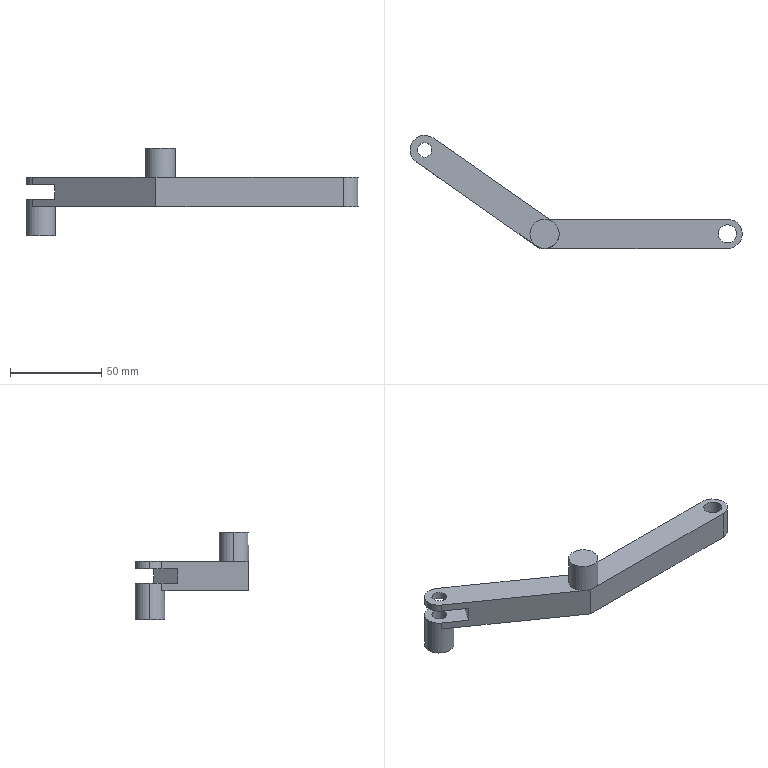Part | SolidWorks | features ICE 5, Extrusion 1 | 1 solid | 25 faces | box 181.532 x 61.886 x 48 mm | volume 50544 mm3 | cylinder 13 | plane 12 | commonest cylinder face diameters 16 x7 8 x4 10 x2
STEP:
#1=CARTESIAN_POINT('',(-169.532,45.886,12.));
#2=VERTEX_POINT('',#1);
#3=CARTESIAN_POINT('',(-161.532,45.886,12.));
#4=VERTEX_POINT('',#3);
#5=CARTESIAN_POINT('',(-165.532,45.886,12.));
#6=DIRECTION('',(0.,0.,1.));
#7=DIRECTION('',(1.,0.,0.));
#8=AXIS2_PLACEMENT_3D('',#5,#6,#7);
#9=CIRCLE('',#8,4.);
#10=EDGE_CURVE('',#2,#4,#9,.T.);
#11=ORIENTED_EDGE('',*,*,#10,.F.);
#12=CARTESIAN_POINT('',(-169.532,45.886,16.));
#13=VERTEX_POINT('',#12);
#14=CARTESIAN_POINT('',(-169.532,45.886,-22.));
#15=DIRECTION('',(0.,0.,1.));
#16=VECTOR('',#15,1000.);
#17=LINE('',#14,#16);
#18=EDGE_CURVE('',#2,#13,#17,.T.);
#19=ORIENTED_EDGE('',*,*,#18,.T.);
#20=CARTESIAN_POINT('',(-161.532,45.886,16.));
#21=VERTEX_POINT('',#20);
#22=CARTESIAN_POINT('',(-165.532,45.886,16.));
#23=DIRECTION('',(0.,0.,1.));
#24=DIRECTION('',(1.,0.,0.));
#25=AXIS2_PLACEMENT_3D('',#22,#23,#24);
#26=CIRCLE('',#25,4.);
#27=EDGE_CURVE('',#13,#21,#26,.T.);
#28=ORIENTED_EDGE('',*,*,#27,.T.);
#29=CARTESIAN_POINT('',(-161.532,45.886,-22.));
#30=DIRECTION('',(0.,0.,1.));
#31=VECTOR('',#30,1000.);
#32=LINE('',#29,#31);
#33=EDGE_CURVE('',#4,#21,#32,.T.);
#34=ORIENTED_EDGE('',*,*,#33,.F.);
#35=EDGE_LOOP('',(#11,#19,#28,#34));
#36=FACE_OUTER_BOUND('',#35,.T.);
#37=CARTESIAN_POINT('',(-165.532,45.886,-22.));
#38=DIRECTION('',(0.,0.,1.));
#39=DIRECTION('',(1.,0.,0.));
#40=AXIS2_PLACEMENT_3D('',#37,#38,#39);
#41=CYLINDRICAL_SURFACE('',#40,4.);
#42=ADVANCED_FACE('',(#36),#41,.F.);
#43=CARTESIAN_POINT('',(-169.532,45.886,-16.));
#44=VERTEX_POINT('',#43);
#45=CARTESIAN_POINT('',(-161.532,45.886,-16.));
#46=VERTEX_POINT('',#45);
#47=CARTESIAN_POINT('',(-165.532,45.886,-16.));
#48=DIRECTION('',(0.,0.,1.));
#49=DIRECTION('',(1.,0.,0.));
#50=AXIS2_PLACEMENT_3D('',#47,#48,#49);
#51=CIRCLE('',#50,4.);
#52=EDGE_CURVE('',#44,#46,#51,.T.);
#53=ORIENTED_EDGE('',*,*,#52,.F.);
#54=CARTESIAN_POINT('',(-169.532,45.886,4.));
#55=VERTEX_POINT('',#54);
#56=CARTESIAN_POINT('',(-169.532,45.886,-22.));
#57=DIRECTION('',(0.,0.,1.));
#58=VECTOR('',#57,1000.);
#59=LINE('',#56,#58);
#60=EDGE_CURVE('',#44,#55,#59,.T.);
#61=ORIENTED_EDGE('',*,*,#60,.T.);
#62=CARTESIAN_POINT('',(-161.532,45.886,4.));
#63=VERTEX_POINT('',#62);
#64=CARTESIAN_POINT('',(-165.532,45.886,4.));
#65=DIRECTION('',(0.,0.,-1.));
#66=DIRECTION('',(-1.,0.,0.));
#67=AXIS2_PLACEMENT_3D('',#64,#65,#66);
#68=CIRCLE('',#67,4.);
#69=EDGE_CURVE('',#63,#55,#68,.T.);
#70=ORIENTED_EDGE('',*,*,#69,.F.);
#71=CARTESIAN_POINT('',(-161.532,45.886,-22.));
#72=DIRECTION('',(0.,0.,1.));
#73=VECTOR('',#72,1000.);
#74=LINE('',#71,#73);
#75=EDGE_CURVE('',#46,#63,#74,.T.);
#76=ORIENTED_EDGE('',*,*,#75,.F.);
#77=EDGE_LOOP('',(#53,#61,#70,#76));
#78=FACE_OUTER_BOUND('',#77,.T.);
#79=CARTESIAN_POINT('',(-165.532,45.886,-22.));
#80=DIRECTION('',(0.,0.,1.));
#81=DIRECTION('',(1.,0.,0.));
#82=AXIS2_PLACEMENT_3D('',#79,#80,#81);
#83=CYLINDRICAL_SURFACE('',#82,4.);
#84=ADVANCED_FACE('',(#78),#83,.F.);
#85=CARTESIAN_POINT('',(-108.,0.,32.));
#86=VERTEX_POINT('',#85);
#87=CARTESIAN_POINT('',(-92.,0.,32.));
#88=VERTEX_POINT('',#87);
#89=CARTESIAN_POINT('',(-100.,0.,32.));
#90=DIRECTION('',(0.,0.,-1.));
#91=DIRECTION('',(-1.,0.,0.));
#92=AXIS2_PLACEMENT_3D('',#89,#90,#91);
#93=CIRCLE('',#92,8.);
#94=EDGE_CURVE('',#86,#88,#93,.T.);
#95=ORIENTED_EDGE('',*,*,#94,.T.);
#96=CARTESIAN_POINT('',(-92.,0.,16.));
#97=VERTEX_POINT('',#96);
#98=CARTESIAN_POINT('',(-92.,0.,32.));
#99=DIRECTION('',(0.,0.,-1.));
#100=VECTOR('',#99,1000.);
#101=LINE('',#98,#100);
#102=EDGE_CURVE('',#88,#97,#101,.T.);
#103=ORIENTED_EDGE('',*,*,#102,.T.);
#104=CARTESIAN_POINT('',(-108.,0.,16.));
#105=VERTEX_POINT('',#104);
#106=CARTESIAN_POINT('',(-100.,0.,16.));
#107=DIRECTION('',(0.,0.,-1.));
#108=DIRECTION('',(-1.,0.,0.));
#109=AXIS2_PLACEMENT_3D('',#106,#107,#108);
#110=CIRCLE('',#109,8.);
#111=EDGE_CURVE('',#105,#97,#110,.T.);
#112=ORIENTED_EDGE('',*,*,#111,.F.);
#113=CARTESIAN_POINT('',(-108.,0.,32.));
#114=DIRECTION('',(0.,0.,-1.));
#115=VECTOR('',#114,1000.);
#116=LINE('',#113,#115);
#117=EDGE_CURVE('',#86,#105,#116,.T.);
#118=ORIENTED_EDGE('',*,*,#117,.F.);
#119=EDGE_LOOP('',(#95,#103,#112,#118));
#120=FACE_OUTER_BOUND('',#119,.T.);
#121=CARTESIAN_POINT('',(-100.,0.,32.));
#122=DIRECTION('',(0.,0.,-1.));
#123=DIRECTION('',(-1.,0.,0.));
#124=AXIS2_PLACEMENT_3D('',#121,#122,#123);
#125=CYLINDRICAL_SURFACE('',#124,8.);
#126=ADVANCED_FACE('',(#120),#125,.T.);
#127=CARTESIAN_POINT('',(-5.,0.,0.));
#128=VERTEX_POINT('',#127);
#129=CARTESIAN_POINT('',(5.,0.,0.));
#130=VERTEX_POINT('',#129);
#131=CARTESIAN_POINT('',(0.,0.,0.));
#132=DIRECTION('',(0.,0.,1.));
#133=DIRECTION('',(1.,0.,0.));
#134=AXIS2_PLACEMENT_3D('',#131,#132,#133);
#135=CIRCLE('',#134,5.);
#136=EDGE_CURVE('',#128,#130,#135,.T.);
#137=ORIENTED_EDGE('',*,*,#136,.F.);
#138=CARTESIAN_POINT('',(-5.,0.,16.));
#139=VERTEX_POINT('',#138);
#140=CARTESIAN_POINT('',(-5.,0.,0.));
#141=DIRECTION('',(0.,0.,1.));
#142=VECTOR('',#141,1000.);
#143=LINE('',#140,#142);
#144=EDGE_CURVE('',#128,#139,#143,.T.);
#145=ORIENTED_EDGE('',*,*,#144,.T.);
#146=CARTESIAN_POINT('',(5.,0.,16.));
#147=VERTEX_POINT('',#146);
#148=CARTESIAN_POINT('',(0.,0.,16.));
#149=DIRECTION('',(0.,0.,1.));
#150=DIRECTION('',(1.,0.,0.));
#151=AXIS2_PLACEMENT_3D('',#148,#149,#150);
#152=CIRCLE('',#151,5.);
#153=EDGE_CURVE('',#139,#147,#152,.T.);
#154=ORIENTED_EDGE('',*,*,#153,.T.);
#155=CARTESIAN_POINT('',(5.,0.,0.));
#156=DIRECTION('',(0.,0.,1.));
#157=VECTOR('',#156,1000.);
#158=LINE('',#155,#157);
#159=EDGE_CURVE('',#130,#147,#158,.T.);
#160=ORIENTED_EDGE('',*,*,#159,.F.);
#161=EDGE_LOOP('',(#137,#145,#154,#160));
#162=FACE_OUTER_BOUND('',#161,.T.);
#163=CARTESIAN_POINT('',(0.,0.,0.));
#164=DIRECTION('',(0.,0.,1.));
#165=DIRECTION('',(1.,0.,0.));
#166=AXIS2_PLACEMENT_3D('',#163,#164,#165);
#167=CYLINDRICAL_SURFACE('',#166,5.);
#168=ADVANCED_FACE('',(#162),#167,.F.);
#169=CARTESIAN_POINT('',(-160.944,52.439,0.));
#170=VERTEX_POINT('',#169);
#171=CARTESIAN_POINT('',(-157.532,45.886,0.));
#172=VERTEX_POINT('',#171);
#173=CARTESIAN_POINT('',(-165.532,45.886,0.));
#174=DIRECTION('',(0.,0.,-1.));
#175=DIRECTION('',(-1.,0.,0.));
#176=AXIS2_PLACEMENT_3D('',#173,#174,#175);
#177=CIRCLE('',#176,8.);
#178=EDGE_CURVE('',#170,#172,#177,.T.);
#179=ORIENTED_EDGE('',*,*,#178,.T.);
#180=CARTESIAN_POINT('',(-157.532,45.886,-16.));
#181=VERTEX_POINT('',#180);
#182=CARTESIAN_POINT('',(-157.532,45.886,16.));
#183=DIRECTION('',(0.,0.,-1.));
#184=VECTOR('',#183,1000.);
#185=LINE('',#182,#184);
#186=EDGE_CURVE('',#172,#181,#185,.T.);
#187=ORIENTED_EDGE('',*,*,#186,.T.);
#188=CARTESIAN_POINT('',(-173.532,45.886,-16.));
#189=VERTEX_POINT('',#188);
#190=CARTESIAN_POINT('',(-165.532,45.886,-16.));
#191=DIRECTION('',(0.,0.,1.));
#192=DIRECTION('',(1.,0.,0.));
#193=AXIS2_PLACEMENT_3D('',#190,#191,#192);
#194=CIRCLE('',#193,8.);
#195=EDGE_CURVE('',#181,#189,#194,.T.);
#196=ORIENTED_EDGE('',*,*,#195,.T.);
#197=CARTESIAN_POINT('',(-173.532,45.886,4.));
#198=VERTEX_POINT('',#197);
#199=CARTESIAN_POINT('',(-173.532,45.886,16.));
#200=DIRECTION('',(0.,0.,-1.));
#201=VECTOR('',#200,1000.);
#202=LINE('',#199,#201);
#203=EDGE_CURVE('',#198,#189,#202,.T.);
#204=ORIENTED_EDGE('',*,*,#203,.F.);
#205=CARTESIAN_POINT('',(-160.944,52.439,4.));
#206=VERTEX_POINT('',#205);
#207=CARTESIAN_POINT('',(-165.532,45.886,4.));
#208=DIRECTION('',(0.,0.,-1.));
#209=DIRECTION('',(-1.,0.,0.));
#210=AXIS2_PLACEMENT_3D('',#207,#208,#209);
#211=CIRCLE('',#210,8.);
#212=EDGE_CURVE('',#198,#206,#211,.T.);
#213=ORIENTED_EDGE('',*,*,#212,.T.);
#214=CARTESIAN_POINT('',(-160.944,52.439,16.));
#215=DIRECTION('',(0.,0.,-1.));
#216=VECTOR('',#215,1000.);
#217=LINE('',#214,#216);
#218=EDGE_CURVE('',#206,#170,#217,.T.);
#219=ORIENTED_EDGE('',*,*,#218,.T.);
#220=EDGE_LOOP('',(#179,#187,#196,#204,#213,#219));
#221=FACE_OUTER_BOUND('',#220,.T.);
#222=CARTESIAN_POINT('',(-165.532,45.886,16.));
#223=DIRECTION('',(0.,0.,-1.));
#224=DIRECTION('',(-1.,0.,0.));
#225=AXIS2_PLACEMENT_3D('',#222,#223,#224);
#226=CYLINDRICAL_SURFACE('',#225,8.);
#227=ADVANCED_FACE('',(#221),#226,.T.);
#228=CARTESIAN_POINT('',(-173.532,45.886,16.));
#229=VERTEX_POINT('',#228);
#230=CARTESIAN_POINT('',(-170.121,39.333,16.));
#231=VERTEX_POINT('',#230);
#232=CARTESIAN_POINT('',(-165.532,45.886,16.));
#233=DIRECTION('',(0.,0.,1.));
#234=DIRECTION('',(1.,0.,0.));
#235=AXIS2_PLACEMENT_3D('',#232,#233,#234);
#236=CIRCLE('',#235,8.);
#237=EDGE_CURVE('',#229,#231,#236,.T.);
#238=ORIENTED_EDGE('',*,*,#237,.F.);
#239=CARTESIAN_POINT('',(-173.532,45.886,12.));
#240=VERTEX_POINT('',#239);
#241=CARTESIAN_POINT('',(-173.532,45.886,16.));
#242=DIRECTION('',(0.,0.,-1.));
#243=VECTOR('',#242,1000.);
#244=LINE('',#241,#243);
#245=EDGE_CURVE('',#229,#240,#244,.T.);
#246=ORIENTED_EDGE('',*,*,#245,.T.);
#247=CARTESIAN_POINT('',(-170.121,39.333,12.));
#248=VERTEX_POINT('',#247);
#249=CARTESIAN_POINT('',(-165.532,45.886,12.));
#250=DIRECTION('',(0.,0.,1.));
#251=DIRECTION('',(1.,0.,0.));
#252=AXIS2_PLACEMENT_3D('',#249,#250,#251);
#253=CIRCLE('',#252,8.);
#254=EDGE_CURVE('',#240,#248,#253,.T.);
#255=ORIENTED_EDGE('',*,*,#254,.T.);
#256=CARTESIAN_POINT('',(-170.121,39.333,16.));
#257=DIRECTION('',(0.,0.,-1.));
#258=VECTOR('',#257,1000.);
#259=LINE('',#256,#258);
#260=EDGE_CURVE('',#231,#248,#259,.T.);
#261=ORIENTED_EDGE('',*,*,#260,.F.);
#262=EDGE_LOOP('',(#238,#246,#255,#261));
#263=FACE_OUTER_BOUND('',#262,.T.);
#264=CARTESIAN_POINT('',(-165.532,45.886,16.));
#265=DIRECTION('',(0.,0.,-1.));
#266=DIRECTION('',(-1.,0.,0.));
#267=AXIS2_PLACEMENT_3D('',#264,#265,#266);
#268=CYLINDRICAL_SURFACE('',#267,8.);
#269=ADVANCED_FACE('',(#263),#268,.T.);
#270=ORIENTED_EDGE('',*,*,#245,.F.);
#271=CARTESIAN_POINT('',(-160.944,52.439,16.));
#272=VERTEX_POINT('',#271);
#273=CARTESIAN_POINT('',(-165.532,45.886,16.));
#274=DIRECTION('',(0.,0.,1.));
#275=DIRECTION('',(1.,0.,0.));
#276=AXIS2_PLACEMENT_3D('',#273,#274,#275);
#277=CIRCLE('',#276,8.);
#278=EDGE_CURVE('',#272,#229,#277,.T.);
#279=ORIENTED_EDGE('',*,*,#278,.F.);
#280=CARTESIAN_POINT('',(-160.944,52.439,12.));
#281=VERTEX_POINT('',#280);
#282=CARTESIAN_POINT('',(-160.944,52.439,16.));
#283=DIRECTION('',(0.,0.,-1.));
#284=VECTOR('',#283,1000.);
#285=LINE('',#282,#284);
#286=EDGE_CURVE('',#272,#281,#285,.T.);
#287=ORIENTED_EDGE('',*,*,#286,.T.);
#288=CARTESIAN_POINT('',(-165.532,45.886,12.));
#289=DIRECTION('',(0.,0.,1.));
#290=DIRECTION('',(1.,0.,0.));
#291=AXIS2_PLACEMENT_3D('',#288,#289,#290);
#292=CIRCLE('',#291,8.);
#293=EDGE_CURVE('',#281,#240,#292,.T.);
#294=ORIENTED_EDGE('',*,*,#293,.T.);
#295=EDGE_LOOP('',(#270,#279,#287,#294));
#296=FACE_OUTER_BOUND('',#295,.T.);
#297=CARTESIAN_POINT('',(-165.532,45.886,16.));
#298=DIRECTION('',(0.,0.,-1.));
#299=DIRECTION('',(-1.,0.,0.));
#300=AXIS2_PLACEMENT_3D('',#297,#298,#299);
#301=CYLINDRICAL_SURFACE('',#300,8.);
#302=ADVANCED_FACE('',(#296),#301,.T.);
#303=CARTESIAN_POINT('',(-102.522,-8.,16.));
#304=VERTEX_POINT('',#303);
#305=CARTESIAN_POINT('',(-100.,-8.,16.));
#306=VERTEX_POINT('',#305);
#307=CARTESIAN_POINT('',(0.,-8.,16.));
#308=DIRECTION('',(1.,0.,0.));
#309=VECTOR('',#308,1000.);
#310=LINE('',#307,#309);
#311=EDGE_CURVE('',#304,#306,#310,.T.);
#312=ORIENTED_EDGE('',*,*,#311,.T.);
#313=CARTESIAN_POINT('',(-104.589,-6.553,16.));
#314=VERTEX_POINT('',#313);
#315=CARTESIAN_POINT('',(-100.,0.,16.));
#316=DIRECTION('',(0.,0.,-1.));
#317=DIRECTION('',(-1.,0.,0.));
#318=AXIS2_PLACEMENT_3D('',#315,#316,#317);
#319=CIRCLE('',#318,8.);
#320=EDGE_CURVE('',#306,#314,#319,.T.);
#321=ORIENTED_EDGE('',*,*,#320,.T.);
#322=CARTESIAN_POINT('',(-102.522,-8.,16.));
#323=DIRECTION('',(0.8192,-0.5736,0.));
#324=VECTOR('',#323,1000.);
#325=LINE('',#322,#324);
#326=EDGE_CURVE('',#314,#304,#325,.T.);
#327=ORIENTED_EDGE('',*,*,#326,.T.);
#328=EDGE_LOOP('',(#312,#321,#327));
#329=FACE_OUTER_BOUND('',#328,.T.);
#330=CARTESIAN_POINT('',(0.,0.,16.));
#331=DIRECTION('',(0.,0.,-1.));
#332=DIRECTION('',(-1.,0.,0.));
#333=AXIS2_PLACEMENT_3D('',#330,#331,#332);
#334=PLANE('',#333);
#335=ADVANCED_FACE('',(#329),#334,.F.);
#336=CARTESIAN_POINT('',(0.,-8.,0.));
#337=VERTEX_POINT('',#336);
#338=CARTESIAN_POINT('',(0.,8.,0.));
#339=VERTEX_POINT('',#338);
#340=CARTESIAN_POINT('',(0.,0.,0.));
#341=DIRECTION('',(0.,0.,1.));
#342=DIRECTION('',(-1.,0.,0.));
#343=AXIS2_PLACEMENT_3D('',#340,#341,#342);
#344=CIRCLE('',#343,8.);
#345=EDGE_CURVE('',#337,#339,#344,.T.);
#346=ORIENTED_EDGE('',*,*,#345,.T.);
#347=CARTESIAN_POINT('',(0.,8.,16.));
#348=VERTEX_POINT('',#347);
#349=CARTESIAN_POINT('',(0.,8.,16.));
#350=DIRECTION('',(0.,0.,-1.));
#351=VECTOR('',#350,1000.);
#352=LINE('',#349,#351);
#353=EDGE_CURVE('',#348,#339,#352,.T.);
#354=ORIENTED_EDGE('',*,*,#353,.F.);
#355=CARTESIAN_POINT('',(0.,-8.,16.));
#356=VERTEX_POINT('',#355);
#357=CARTESIAN_POINT('',(0.,0.,16.));
#358=DIRECTION('',(0.,0.,1.));
#359=DIRECTION('',(-1.,0.,0.));
#360=AXIS2_PLACEMENT_3D('',#357,#358,#359);
#361=CIRCLE('',#360,8.);
#362=EDGE_CURVE('',#356,#348,#361,.T.);
#363=ORIENTED_EDGE('',*,*,#362,.F.);
#364=CARTESIAN_POINT('',(0.,-8.,16.));
#365=DIRECTION('',(0.,0.,-1.));
#366=VECTOR('',#365,1000.);
#367=LINE('',#364,#366);
#368=EDGE_CURVE('',#356,#337,#367,.T.);
#369=ORIENTED_EDGE('',*,*,#368,.T.);
#370=EDGE_LOOP('',(#346,#354,#363,#369));
#371=FACE_OUTER_BOUND('',#370,.T.);
#372=CARTESIAN_POINT('',(0.,0.,16.));
#373=DIRECTION('',(0.,0.,-1.));
#374=DIRECTION('',(-1.,0.,0.));
#375=AXIS2_PLACEMENT_3D('',#372,#373,#374);
#376=CYLINDRICAL_SURFACE('',#375,8.);
#377=ADVANCED_FACE('',(#371),#376,.T.);
#378=CARTESIAN_POINT('',(-97.478,8.,0.));
#379=VERTEX_POINT('',#378);
#380=CARTESIAN_POINT('',(0.,8.,0.));
#381=DIRECTION('',(-1.,0.,0.));
#382=VECTOR('',#381,1000.);
#383=LINE('',#380,#382);
#384=EDGE_CURVE('',#339,#379,#383,.T.);
#385=ORIENTED_EDGE('',*,*,#384,.T.);
#386=CARTESIAN_POINT('',(-97.478,8.,16.));
#387=VERTEX_POINT('',#386);
#388=CARTESIAN_POINT('',(-97.478,8.,16.));
#389=DIRECTION('',(0.,0.,-1.));
#390=VECTOR('',#389,1000.);
#391=LINE('',#388,#390);
#392=EDGE_CURVE('',#387,#379,#391,.T.);
#393=ORIENTED_EDGE('',*,*,#392,.F.);
#394=CARTESIAN_POINT('',(0.,8.,16.));
#395=DIRECTION('',(-1.,0.,0.));
#396=VECTOR('',#395,1000.);
#397=LINE('',#394,#396);
#398=EDGE_CURVE('',#348,#387,#397,.T.);
#399=ORIENTED_EDGE('',*,*,#398,.F.);
#400=ORIENTED_EDGE('',*,*,#353,.T.);
#401=EDGE_LOOP('',(#385,#393,#399,#400));
#402=FACE_OUTER_BOUND('',#401,.T.);
#403=CARTESIAN_POINT('',(0.,8.,16.));
#404=DIRECTION('',(0.,-1.,0.));
#405=DIRECTION('',(0.,0.,-1.));
#406=AXIS2_PLACEMENT_3D('',#403,#404,#405);
#407=PLANE('',#406);
#408=ADVANCED_FACE('',(#402),#407,.F.);
#409=CARTESIAN_POINT('',(-148.656,43.836,4.));
#410=VERTEX_POINT('',#409);
#411=CARTESIAN_POINT('',(-148.656,43.836,12.));
#412=VERTEX_POINT('',#411);
#413=CARTESIAN_POINT('',(-148.656,43.836,16.));
#414=DIRECTION('',(0.,0.,1.));
#415=VECTOR('',#414,1000.);
#416=LINE('',#413,#415);
#417=EDGE_CURVE('',#410,#412,#416,.T.);
#418=ORIENTED_EDGE('',*,*,#417,.T.);
#419=CARTESIAN_POINT('',(-97.478,8.,12.));
#420=DIRECTION('',(-0.8192,0.5736,0.));
#421=VECTOR('',#420,1000.);
#422=LINE('',#419,#421);
#423=EDGE_CURVE('',#412,#281,#422,.T.);
#424=ORIENTED_EDGE('',*,*,#423,.T.);
#425=ORIENTED_EDGE('',*,*,#286,.F.);
#426=CARTESIAN_POINT('',(-97.478,8.,16.));
#427=DIRECTION('',(-0.8192,0.5736,0.));
#428=VECTOR('',#427,1000.);
#429=LINE('',#426,#428);
#430=EDGE_CURVE('',#387,#272,#429,.T.);
#431=ORIENTED_EDGE('',*,*,#430,.F.);
#432=ORIENTED_EDGE('',*,*,#392,.T.);
#433=CARTESIAN_POINT('',(-97.478,8.,0.));
#434=DIRECTION('',(-0.8192,0.5736,0.));
#435=VECTOR('',#434,1000.);
#436=LINE('',#433,#435);
#437=EDGE_CURVE('',#379,#170,#436,.T.);
#438=ORIENTED_EDGE('',*,*,#437,.T.);
#439=ORIENTED_EDGE('',*,*,#218,.F.);
#440=CARTESIAN_POINT('',(-97.478,8.,4.));
#441=DIRECTION('',(0.8192,-0.5736,0.));
#442=VECTOR('',#441,1000.);
#443=LINE('',#440,#442);
#444=EDGE_CURVE('',#206,#410,#443,.T.);
#445=ORIENTED_EDGE('',*,*,#444,.T.);
#446=EDGE_LOOP('',(#418,#424,#425,#431,#432,#438,#439,#445));
#447=FACE_OUTER_BOUND('',#446,.T.);
#448=CARTESIAN_POINT('',(-97.478,8.,16.));
#449=DIRECTION('',(-0.5736,-0.8192,0.));
#450=DIRECTION('',(0.8192,-0.5736,0.));
#451=AXIS2_PLACEMENT_3D('',#448,#449,#450);
#452=PLANE('',#451);
#453=ADVANCED_FACE('',(#447),#452,.F.);
#454=ORIENTED_EDGE('',*,*,#186,.F.);
#455=CARTESIAN_POINT('',(-170.121,39.333,0.));
#456=VERTEX_POINT('',#455);
#457=CARTESIAN_POINT('',(-165.532,45.886,0.));
#458=DIRECTION('',(0.,0.,-1.));
#459=DIRECTION('',(-1.,0.,0.));
#460=AXIS2_PLACEMENT_3D('',#457,#458,#459);
#461=CIRCLE('',#460,8.);
#462=EDGE_CURVE('',#172,#456,#461,.T.);
#463=ORIENTED_EDGE('',*,*,#462,.T.);
#464=CARTESIAN_POINT('',(-170.121,39.333,4.));
#465=VERTEX_POINT('',#464);
#466=CARTESIAN_POINT('',(-170.121,39.333,16.));
#467=DIRECTION('',(0.,0.,-1.));
#468=VECTOR('',#467,1000.);
#469=LINE('',#466,#468);
#470=EDGE_CURVE('',#465,#456,#469,.T.);
#471=ORIENTED_EDGE('',*,*,#470,.F.);
#472=CARTESIAN_POINT('',(-165.532,45.886,4.));
#473=DIRECTION('',(0.,0.,-1.));
#474=DIRECTION('',(-1.,0.,0.));
#475=AXIS2_PLACEMENT_3D('',#472,#473,#474);
#476=CIRCLE('',#475,8.);
#477=EDGE_CURVE('',#465,#198,#476,.T.);
#478=ORIENTED_EDGE('',*,*,#477,.T.);
#479=ORIENTED_EDGE('',*,*,#203,.T.);
#480=CARTESIAN_POINT('',(-165.532,45.886,-16.));
#481=DIRECTION('',(0.,0.,1.));
#482=DIRECTION('',(1.,0.,0.));
#483=AXIS2_PLACEMENT_3D('',#480,#481,#482);
#484=CIRCLE('',#483,8.);
#485=EDGE_CURVE('',#189,#181,#484,.T.);
#486=ORIENTED_EDGE('',*,*,#485,.T.);
#487=EDGE_LOOP('',(#454,#463,#471,#478,#479,#486));
#488=FACE_OUTER_BOUND('',#487,.T.);
#489=CARTESIAN_POINT('',(-165.532,45.886,16.));
#490=DIRECTION('',(0.,0.,-1.));
#491=DIRECTION('',(-1.,0.,0.));
#492=AXIS2_PLACEMENT_3D('',#489,#490,#491);
#493=CYLINDRICAL_SURFACE('',#492,8.);
#494=ADVANCED_FACE('',(#488),#493,.T.);
#495=ORIENTED_EDGE('',*,*,#260,.T.);
#496=CARTESIAN_POINT('',(-157.833,30.729,12.));
#497=VERTEX_POINT('',#496);
#498=CARTESIAN_POINT('',(-157.833,30.729,12.));
#499=DIRECTION('',(-0.8192,0.5736,0.));
#500=VECTOR('',#499,1000.);
#501=LINE('',#498,#500);
#502=EDGE_CURVE('',#497,#248,#501,.T.);
#503=ORIENTED_EDGE('',*,*,#502,.F.);
#504=CARTESIAN_POINT('',(-157.833,30.729,4.));
#505=VERTEX_POINT('',#504);
#506=CARTESIAN_POINT('',(-157.833,30.729,4.));
#507=DIRECTION('',(0.,0.,1.));
#508=VECTOR('',#507,1000.);
#509=LINE('',#506,#508);
#510=EDGE_CURVE('',#505,#497,#509,.T.);
#511=ORIENTED_EDGE('',*,*,#510,.F.);
#512=CARTESIAN_POINT('',(-102.522,-8.,4.));
#513=DIRECTION('',(-0.8192,0.5736,0.));
#514=VECTOR('',#513,1000.);
#515=LINE('',#512,#514);
#516=EDGE_CURVE('',#505,#465,#515,.T.);
#517=ORIENTED_EDGE('',*,*,#516,.T.);
#518=ORIENTED_EDGE('',*,*,#470,.T.);
#519=CARTESIAN_POINT('',(-102.522,-8.,0.));
#520=VERTEX_POINT('',#519);
#521=CARTESIAN_POINT('',(-102.522,-8.,0.));
#522=DIRECTION('',(0.8192,-0.5736,0.));
#523=VECTOR('',#522,1000.);
#524=LINE('',#521,#523);
#525=EDGE_CURVE('',#456,#520,#524,.T.);
#526=ORIENTED_EDGE('',*,*,#525,.T.);
#527=CARTESIAN_POINT('',(-102.522,-8.,16.));
#528=DIRECTION('',(0.,0.,-1.));
#529=VECTOR('',#528,1000.);
#530=LINE('',#527,#529);
#531=EDGE_CURVE('',#304,#520,#530,.T.);
#532=ORIENTED_EDGE('',*,*,#531,.F.);
#533=ORIENTED_EDGE('',*,*,#326,.F.);
#534=CARTESIAN_POINT('',(-102.522,-8.,16.));
#535=DIRECTION('',(0.8192,-0.5736,0.));
#536=VECTOR('',#535,1000.);
#537=LINE('',#534,#536);
#538=EDGE_CURVE('',#231,#314,#537,.T.);
#539=ORIENTED_EDGE('',*,*,#538,.F.);
#540=EDGE_LOOP('',(#495,#503,#511,#517,#518,#526,#532,#533,#539));
#541=FACE_OUTER_BOUND('',#540,.T.);
#542=CARTESIAN_POINT('',(-102.522,-8.,16.));
#543=DIRECTION('',(0.5736,0.8192,0.));
#544=DIRECTION('',(-0.8192,0.5736,0.));
#545=AXIS2_PLACEMENT_3D('',#542,#543,#544);
#546=PLANE('',#545);
#547=ADVANCED_FACE('',(#541),#546,.F.);
#548=CARTESIAN_POINT('',(0.,-8.,16.));
#549=DIRECTION('',(1.,0.,0.));
#550=VECTOR('',#549,1000.);
#551=LINE('',#548,#550);
#552=EDGE_CURVE('',#306,#356,#551,.T.);
#553=ORIENTED_EDGE('',*,*,#552,.F.);
#554=ORIENTED_EDGE('',*,*,#311,.F.);
#555=ORIENTED_EDGE('',*,*,#531,.T.);
#556=CARTESIAN_POINT('',(0.,-8.,0.));
#557=DIRECTION('',(1.,0.,0.));
#558=VECTOR('',#557,1000.);
#559=LINE('',#556,#558);
#560=EDGE_CURVE('',#520,#337,#559,.T.);
#561=ORIENTED_EDGE('',*,*,#560,.T.);
#562=ORIENTED_EDGE('',*,*,#368,.F.);
#563=EDGE_LOOP('',(#553,#554,#555,#561,#562));
#564=FACE_OUTER_BOUND('',#563,.T.);
#565=CARTESIAN_POINT('',(0.,-8.,16.));
#566=DIRECTION('',(0.,1.,0.));
#567=DIRECTION('',(0.,0.,1.));
#568=AXIS2_PLACEMENT_3D('',#565,#566,#567);
#569=PLANE('',#568);
#570=ADVANCED_FACE('',(#564),#569,.F.);
#571=CARTESIAN_POINT('',(-165.532,45.886,16.));
#572=DIRECTION('',(0.,0.,1.));
#573=DIRECTION('',(1.,0.,0.));
#574=AXIS2_PLACEMENT_3D('',#571,#572,#573);
#575=CIRCLE('',#574,4.);
#576=EDGE_CURVE('',#21,#13,#575,.T.);
#577=ORIENTED_EDGE('',*,*,#576,.F.);
#578=ORIENTED_EDGE('',*,*,#27,.F.);
#579=EDGE_LOOP('',(#577,#578));
#580=FACE_BOUND('',#579,.T.);
#581=CARTESIAN_POINT('',(0.,0.,16.));
#582=DIRECTION('',(0.,0.,1.));
#583=DIRECTION('',(1.,0.,0.));
#584=AXIS2_PLACEMENT_3D('',#581,#582,#583);
#585=CIRCLE('',#584,5.);
#586=EDGE_CURVE('',#147,#139,#585,.T.);
#587=ORIENTED_EDGE('',*,*,#586,.F.);
#588=ORIENTED_EDGE('',*,*,#153,.F.);
#589=EDGE_LOOP('',(#587,#588));
#590=FACE_BOUND('',#589,.T.);
#591=ORIENTED_EDGE('',*,*,#430,.T.);
#592=ORIENTED_EDGE('',*,*,#278,.T.);
#593=ORIENTED_EDGE('',*,*,#237,.T.);
#594=ORIENTED_EDGE('',*,*,#538,.T.);
#595=CARTESIAN_POINT('',(-100.,0.,16.));
#596=DIRECTION('',(0.,0.,-1.));
#597=DIRECTION('',(-1.,0.,0.));
#598=AXIS2_PLACEMENT_3D('',#595,#596,#597);
#599=CIRCLE('',#598,8.);
#600=EDGE_CURVE('',#314,#105,#599,.T.);
#601=ORIENTED_EDGE('',*,*,#600,.T.);
#602=ORIENTED_EDGE('',*,*,#111,.T.);
#603=CARTESIAN_POINT('',(-100.,0.,16.));
#604=DIRECTION('',(0.,0.,-1.));
#605=DIRECTION('',(-1.,0.,0.));
#606=AXIS2_PLACEMENT_3D('',#603,#604,#605);
#607=CIRCLE('',#606,8.);
#608=EDGE_CURVE('',#97,#306,#607,.T.);
#609=ORIENTED_EDGE('',*,*,#608,.T.);
#610=ORIENTED_EDGE('',*,*,#552,.T.);
#611=ORIENTED_EDGE('',*,*,#362,.T.);
#612=ORIENTED_EDGE('',*,*,#398,.T.);
#613=EDGE_LOOP('',(#591,#592,#593,#594,#601,#602,#609,#610,#611,#612));
#614=FACE_OUTER_BOUND('',#613,.T.);
#615=CARTESIAN_POINT('',(0.,0.,16.));
#616=DIRECTION('',(0.,0.,-1.));
#617=DIRECTION('',(-1.,0.,0.));
#618=AXIS2_PLACEMENT_3D('',#615,#616,#617);
#619=PLANE('',#618);
#620=ADVANCED_FACE('',(#580,#590,#614),#619,.F.);
#621=ORIENTED_EDGE('',*,*,#178,.F.);
#622=ORIENTED_EDGE('',*,*,#437,.F.);
#623=ORIENTED_EDGE('',*,*,#384,.F.);
#624=ORIENTED_EDGE('',*,*,#345,.F.);
#625=ORIENTED_EDGE('',*,*,#560,.F.);
#626=ORIENTED_EDGE('',*,*,#525,.F.);
#627=ORIENTED_EDGE('',*,*,#462,.F.);
#628=EDGE_LOOP('',(#621,#622,#623,#624,#625,#626,#627));
#629=FACE_OUTER_BOUND('',#628,.T.);
#630=CARTESIAN_POINT('',(0.,0.,0.));
#631=DIRECTION('',(0.,0.,1.));
#632=DIRECTION('',(1.,0.,0.));
#633=AXIS2_PLACEMENT_3D('',#630,#631,#632);
#634=CIRCLE('',#633,5.);
#635=EDGE_CURVE('',#130,#128,#634,.T.);
#636=ORIENTED_EDGE('',*,*,#635,.T.);
#637=ORIENTED_EDGE('',*,*,#136,.T.);
#638=EDGE_LOOP('',(#636,#637));
#639=FACE_BOUND('',#638,.T.);
#640=CARTESIAN_POINT('',(0.,0.,0.));
#641=DIRECTION('',(0.,0.,-1.));
#642=DIRECTION('',(-1.,0.,0.));
#643=AXIS2_PLACEMENT_3D('',#640,#641,#642);
#644=PLANE('',#643);
#645=ADVANCED_FACE('',(#629,#639),#644,.T.);
#646=ORIENTED_EDGE('',*,*,#144,.F.);
#647=ORIENTED_EDGE('',*,*,#635,.F.);
#648=ORIENTED_EDGE('',*,*,#159,.T.);
#649=ORIENTED_EDGE('',*,*,#586,.T.);
#650=EDGE_LOOP('',(#646,#647,#648,#649));
#651=FACE_OUTER_BOUND('',#650,.T.);
#652=CARTESIAN_POINT('',(0.,0.,0.));
#653=DIRECTION('',(0.,0.,1.));
#654=DIRECTION('',(1.,0.,0.));
#655=AXIS2_PLACEMENT_3D('',#652,#653,#654);
#656=CYLINDRICAL_SURFACE('',#655,5.);
#657=ADVANCED_FACE('',(#651),#656,.F.);
#658=ORIENTED_EDGE('',*,*,#102,.F.);
#659=CARTESIAN_POINT('',(-100.,0.,32.));
#660=DIRECTION('',(0.,0.,-1.));
#661=DIRECTION('',(-1.,0.,0.));
#662=AXIS2_PLACEMENT_3D('',#659,#660,#661);
#663=CIRCLE('',#662,8.);
#664=EDGE_CURVE('',#88,#86,#663,.T.);
#665=ORIENTED_EDGE('',*,*,#664,.T.);
#666=ORIENTED_EDGE('',*,*,#117,.T.);
#667=ORIENTED_EDGE('',*,*,#600,.F.);
#668=ORIENTED_EDGE('',*,*,#320,.F.);
#669=ORIENTED_EDGE('',*,*,#608,.F.);
#670=EDGE_LOOP('',(#658,#665,#666,#667,#668,#669));
#671=FACE_OUTER_BOUND('',#670,.T.);
#672=CARTESIAN_POINT('',(-100.,0.,32.));
#673=DIRECTION('',(0.,0.,-1.));
#674=DIRECTION('',(-1.,0.,0.));
#675=AXIS2_PLACEMENT_3D('',#672,#673,#674);
#676=CYLINDRICAL_SURFACE('',#675,8.);
#677=ADVANCED_FACE('',(#671),#676,.T.);
#678=ORIENTED_EDGE('',*,*,#94,.F.);
#679=ORIENTED_EDGE('',*,*,#664,.F.);
#680=EDGE_LOOP('',(#678,#679));
#681=FACE_OUTER_BOUND('',#680,.T.);
#682=CARTESIAN_POINT('',(-100.,0.,32.));
#683=DIRECTION('',(0.,0.,-1.));
#684=DIRECTION('',(-1.,0.,0.));
#685=AXIS2_PLACEMENT_3D('',#682,#683,#684);
#686=PLANE('',#685);
#687=ADVANCED_FACE('',(#681),#686,.F.);
#688=CARTESIAN_POINT('',(-165.532,45.886,-16.));
#689=DIRECTION('',(0.,0.,1.));
#690=DIRECTION('',(1.,0.,0.));
#691=AXIS2_PLACEMENT_3D('',#688,#689,#690);
#692=CIRCLE('',#691,4.);
#693=EDGE_CURVE('',#46,#44,#692,.T.);
#694=ORIENTED_EDGE('',*,*,#693,.T.);
#695=ORIENTED_EDGE('',*,*,#52,.T.);
#696=EDGE_LOOP('',(#694,#695));
#697=FACE_BOUND('',#696,.T.);
#698=ORIENTED_EDGE('',*,*,#485,.F.);
#699=ORIENTED_EDGE('',*,*,#195,.F.);
#700=EDGE_LOOP('',(#698,#699));
#701=FACE_OUTER_BOUND('',#700,.T.);
#702=CARTESIAN_POINT('',(-165.532,45.886,-16.));
#703=DIRECTION('',(0.,0.,1.));
#704=DIRECTION('',(1.,0.,0.));
#705=AXIS2_PLACEMENT_3D('',#702,#703,#704);
#706=PLANE('',#705);
#707=ADVANCED_FACE('',(#697,#701),#706,.F.);
#708=CARTESIAN_POINT('',(-165.532,45.886,12.));
#709=DIRECTION('',(0.,0.,1.));
#710=DIRECTION('',(1.,0.,0.));
#711=AXIS2_PLACEMENT_3D('',#708,#709,#710);
#712=CIRCLE('',#711,4.);
#713=EDGE_CURVE('',#4,#2,#712,.T.);
#714=ORIENTED_EDGE('',*,*,#713,.T.);
#715=ORIENTED_EDGE('',*,*,#10,.T.);
#716=EDGE_LOOP('',(#714,#715));
#717=FACE_BOUND('',#716,.T.);
#718=CARTESIAN_POINT('',(-136.038,61.857,12.));
#719=DIRECTION('',(-0.5736,-0.8192,0.));
#720=VECTOR('',#719,1000.);
#721=LINE('',#718,#720);
#722=EDGE_CURVE('',#412,#497,#721,.T.);
#723=ORIENTED_EDGE('',*,*,#722,.T.);
#724=ORIENTED_EDGE('',*,*,#502,.T.);
#725=ORIENTED_EDGE('',*,*,#254,.F.);
#726=ORIENTED_EDGE('',*,*,#293,.F.);
#727=ORIENTED_EDGE('',*,*,#423,.F.);
#728=EDGE_LOOP('',(#723,#724,#725,#726,#727));
#729=FACE_OUTER_BOUND('',#728,.T.);
#730=CARTESIAN_POINT('',(-136.038,61.857,12.));
#731=DIRECTION('',(0.,0.,1.));
#732=DIRECTION('',(1.,0.,0.));
#733=AXIS2_PLACEMENT_3D('',#730,#731,#732);
#734=PLANE('',#733);
#735=ADVANCED_FACE('',(#717,#729),#734,.F.);
#736=CARTESIAN_POINT('',(-136.038,61.857,4.));
#737=DIRECTION('',(-0.5736,-0.8192,0.));
#738=VECTOR('',#737,1000.);
#739=LINE('',#736,#738);
#740=EDGE_CURVE('',#410,#505,#739,.T.);
#741=ORIENTED_EDGE('',*,*,#740,.T.);
#742=ORIENTED_EDGE('',*,*,#510,.T.);
#743=ORIENTED_EDGE('',*,*,#722,.F.);
#744=ORIENTED_EDGE('',*,*,#417,.F.);
#745=EDGE_LOOP('',(#741,#742,#743,#744));
#746=FACE_OUTER_BOUND('',#745,.T.);
#747=CARTESIAN_POINT('',(-136.038,61.857,4.));
#748=DIRECTION('',(0.8192,-0.5736,0.));
#749=DIRECTION('',(0.5736,0.8192,0.));
#750=AXIS2_PLACEMENT_3D('',#747,#748,#749);
#751=PLANE('',#750);
#752=ADVANCED_FACE('',(#746),#751,.F.);
#753=ORIENTED_EDGE('',*,*,#69,.T.);
#754=CARTESIAN_POINT('',(-165.532,45.886,4.));
#755=DIRECTION('',(0.,0.,-1.));
#756=DIRECTION('',(-1.,0.,0.));
#757=AXIS2_PLACEMENT_3D('',#754,#755,#756);
#758=CIRCLE('',#757,4.);
#759=EDGE_CURVE('',#55,#63,#758,.T.);
#760=ORIENTED_EDGE('',*,*,#759,.T.);
#761=EDGE_LOOP('',(#753,#760));
#762=FACE_BOUND('',#761,.T.);
#763=ORIENTED_EDGE('',*,*,#477,.F.);
#764=ORIENTED_EDGE('',*,*,#516,.F.);
#765=ORIENTED_EDGE('',*,*,#740,.F.);
#766=ORIENTED_EDGE('',*,*,#444,.F.);
#767=ORIENTED_EDGE('',*,*,#212,.F.);
#768=EDGE_LOOP('',(#763,#764,#765,#766,#767));
#769=FACE_OUTER_BOUND('',#768,.T.);
#770=CARTESIAN_POINT('',(-136.038,61.857,4.));
#771=DIRECTION('',(0.,0.,-1.));
#772=DIRECTION('',(-1.,0.,0.));
#773=AXIS2_PLACEMENT_3D('',#770,#771,#772);
#774=PLANE('',#773);
#775=ADVANCED_FACE('',(#762,#769),#774,.F.);
#776=ORIENTED_EDGE('',*,*,#60,.F.);
#777=ORIENTED_EDGE('',*,*,#693,.F.);
#778=ORIENTED_EDGE('',*,*,#75,.T.);
#779=ORIENTED_EDGE('',*,*,#759,.F.);
#780=EDGE_LOOP('',(#776,#777,#778,#779));
#781=FACE_OUTER_BOUND('',#780,.T.);
#782=CARTESIAN_POINT('',(-165.532,45.886,-22.));
#783=DIRECTION('',(0.,0.,1.));
#784=DIRECTION('',(1.,0.,0.));
#785=AXIS2_PLACEMENT_3D('',#782,#783,#784);
#786=CYLINDRICAL_SURFACE('',#785,4.);
#787=ADVANCED_FACE('',(#781),#786,.F.);
#788=ORIENTED_EDGE('',*,*,#18,.F.);
#789=ORIENTED_EDGE('',*,*,#713,.F.);
#790=ORIENTED_EDGE('',*,*,#33,.T.);
#791=ORIENTED_EDGE('',*,*,#576,.T.);
#792=EDGE_LOOP('',(#788,#789,#790,#791));
#793=FACE_OUTER_BOUND('',#792,.T.);
#794=CARTESIAN_POINT('',(-165.532,45.886,-22.));
#795=DIRECTION('',(0.,0.,1.));
#796=DIRECTION('',(1.,0.,0.));
#797=AXIS2_PLACEMENT_3D('',#794,#795,#796);
#798=CYLINDRICAL_SURFACE('',#797,4.);
#799=ADVANCED_FACE('',(#793),#798,.F.);
#800=CLOSED_SHELL('',(#42,#84,#126,#168,#227,#269,#302,#335,#377,#408,#453,#494,#547,#570,#620,#645,#657,#677,#687,#707,#735,#752,#775,#787,#799));
#801=MANIFOLD_SOLID_BREP('',#800);
#802=CARTESIAN_POINT('',(0.,0.,0.));
#803=DIRECTION('',(0.,0.,1.));
#804=DIRECTION('',(1.,0.,0.));
#805=AXIS2_PLACEMENT_3D('',#802,#803,#804);
#806=(LENGTH_UNIT()NAMED_UNIT(*)SI_UNIT(.MILLI.,.METRE.));
#807=UNCERTAINTY_MEASURE_WITH_UNIT(LENGTH_MEASURE(0.00001),#806,'','');
#808=(NAMED_UNIT(*)PLANE_ANGLE_UNIT()SI_UNIT($,.RADIAN.));
#809=(NAMED_UNIT(*)SI_UNIT($,.STERADIAN.)SOLID_ANGLE_UNIT());
#810=(GEOMETRIC_REPRESENTATION_CONTEXT(3)GLOBAL_UNCERTAINTY_ASSIGNED_CONTEXT((#807))GLOBAL_UNIT_ASSIGNED_CONTEXT((#806,#808,#809))REPRESENTATION_CONTEXT('',''));
#811=ADVANCED_BREP_SHAPE_REPRESENTATION('',(#801,#805),#810);